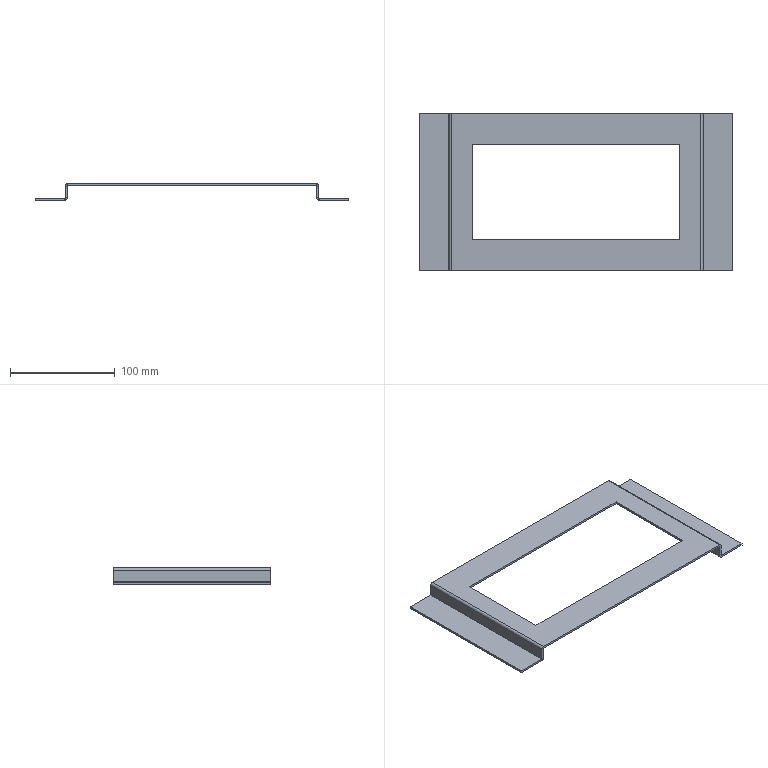Part | 1 solid | 42 faces | box 298 x 150 x 15.5 mm | volume 61242 mm3 | plane 34 | cylinder 8 | commonest cylinder face diameters 0.4 x4 4.4 x4
STEP:
#1=CARTESIAN_POINT('',(121.,75.,-2.2));
#2=VERTEX_POINT('',#1);
#3=CARTESIAN_POINT('',(121.,75.,-13.3));
#4=VERTEX_POINT('',#3);
#5=CARTESIAN_POINT('',(121.,75.,-2.));
#6=DIRECTION('',(0.,0.,-1.));
#7=VECTOR('',#6,1000.);
#8=LINE('',#5,#7);
#9=EDGE_CURVE('',#2,#4,#8,.T.);
#10=ORIENTED_EDGE('',*,*,#9,.T.);
#11=CARTESIAN_POINT('',(119.,75.,-13.3));
#12=VERTEX_POINT('',#11);
#13=CARTESIAN_POINT('',(121.,75.,-13.3));
#14=DIRECTION('',(-1.,0.,0.));
#15=VECTOR('',#14,1000.);
#16=LINE('',#13,#15);
#17=EDGE_CURVE('',#4,#12,#16,.T.);
#18=ORIENTED_EDGE('',*,*,#17,.T.);
#19=CARTESIAN_POINT('',(119.,75.,-2.2));
#20=VERTEX_POINT('',#19);
#21=CARTESIAN_POINT('',(119.,75.,0.));
#22=DIRECTION('',(0.,0.,-1.));
#23=VECTOR('',#22,1000.);
#24=LINE('',#21,#23);
#25=EDGE_CURVE('',#20,#12,#24,.T.);
#26=ORIENTED_EDGE('',*,*,#25,.F.);
#27=CARTESIAN_POINT('',(121.,75.,-2.2));
#28=DIRECTION('',(1.,0.,0.));
#29=VECTOR('',#28,1000.);
#30=LINE('',#27,#29);
#31=EDGE_CURVE('',#20,#2,#30,.T.);
#32=ORIENTED_EDGE('',*,*,#31,.T.);
#33=EDGE_LOOP('',(#10,#18,#26,#32));
#34=FACE_OUTER_BOUND('',#33,.T.);
#35=CARTESIAN_POINT('',(121.,75.,-2.));
#36=DIRECTION('',(0.,1.,0.));
#37=DIRECTION('',(0.,0.,1.));
#38=AXIS2_PLACEMENT_3D('',#35,#36,#37);
#39=PLANE('',#38);
#40=ADVANCED_FACE('',(#34),#39,.T.);
#41=CARTESIAN_POINT('',(121.,-75.,-13.3));
#42=VERTEX_POINT('',#41);
#43=CARTESIAN_POINT('',(121.,75.,-13.3));
#44=DIRECTION('',(0.,-1.,0.));
#45=VECTOR('',#44,1000.);
#46=LINE('',#43,#45);
#47=EDGE_CURVE('',#4,#42,#46,.T.);
#48=ORIENTED_EDGE('',*,*,#47,.F.);
#49=ORIENTED_EDGE('',*,*,#9,.F.);
#50=CARTESIAN_POINT('',(121.,-75.,-2.2));
#51=VERTEX_POINT('',#50);
#52=CARTESIAN_POINT('',(121.,75.,-2.2));
#53=DIRECTION('',(0.,1.,0.));
#54=VECTOR('',#53,1000.);
#55=LINE('',#52,#54);
#56=EDGE_CURVE('',#51,#2,#55,.T.);
#57=ORIENTED_EDGE('',*,*,#56,.F.);
#58=CARTESIAN_POINT('',(121.,-75.,-15.5));
#59=DIRECTION('',(0.,0.,1.));
#60=VECTOR('',#59,1000.);
#61=LINE('',#58,#60);
#62=EDGE_CURVE('',#42,#51,#61,.T.);
#63=ORIENTED_EDGE('',*,*,#62,.F.);
#64=EDGE_LOOP('',(#48,#49,#57,#63));
#65=FACE_OUTER_BOUND('',#64,.T.);
#66=CARTESIAN_POINT('',(121.,0.,0.));
#67=DIRECTION('',(-1.,0.,0.));
#68=DIRECTION('',(0.,0.,1.));
#69=AXIS2_PLACEMENT_3D('',#66,#67,#68);
#70=PLANE('',#69);
#71=ADVANCED_FACE('',(#65),#70,.F.);
#72=ORIENTED_EDGE('',*,*,#25,.T.);
#73=CARTESIAN_POINT('',(119.,-75.,-13.3));
#74=VERTEX_POINT('',#73);
#75=CARTESIAN_POINT('',(119.,75.,-13.3));
#76=DIRECTION('',(0.,-1.,0.));
#77=VECTOR('',#76,1000.);
#78=LINE('',#75,#77);
#79=EDGE_CURVE('',#12,#74,#78,.T.);
#80=ORIENTED_EDGE('',*,*,#79,.T.);
#81=CARTESIAN_POINT('',(119.,-75.,-2.2));
#82=VERTEX_POINT('',#81);
#83=CARTESIAN_POINT('',(119.,-75.,0.));
#84=DIRECTION('',(0.,0.,1.));
#85=VECTOR('',#84,1000.);
#86=LINE('',#83,#85);
#87=EDGE_CURVE('',#74,#82,#86,.T.);
#88=ORIENTED_EDGE('',*,*,#87,.T.);
#89=CARTESIAN_POINT('',(119.,75.,-2.2));
#90=DIRECTION('',(0.,-1.,0.));
#91=VECTOR('',#90,1000.);
#92=LINE('',#89,#91);
#93=EDGE_CURVE('',#20,#82,#92,.T.);
#94=ORIENTED_EDGE('',*,*,#93,.F.);
#95=EDGE_LOOP('',(#72,#80,#88,#94));
#96=FACE_OUTER_BOUND('',#95,.T.);
#97=CARTESIAN_POINT('',(119.,0.,0.));
#98=DIRECTION('',(-1.,0.,0.));
#99=DIRECTION('',(0.,0.,1.));
#100=AXIS2_PLACEMENT_3D('',#97,#98,#99);
#101=PLANE('',#100);
#102=ADVANCED_FACE('',(#96),#101,.T.);
#103=CARTESIAN_POINT('',(-121.,-75.,-2.2));
#104=VERTEX_POINT('',#103);
#105=CARTESIAN_POINT('',(-121.,-75.,-13.3));
#106=VERTEX_POINT('',#105);
#107=CARTESIAN_POINT('',(-121.,-75.,-15.5));
#108=DIRECTION('',(0.,0.,-1.));
#109=VECTOR('',#108,1000.);
#110=LINE('',#107,#109);
#111=EDGE_CURVE('',#104,#106,#110,.T.);
#112=ORIENTED_EDGE('',*,*,#111,.T.);
#113=CARTESIAN_POINT('',(-119.,-75.,-13.3));
#114=VERTEX_POINT('',#113);
#115=CARTESIAN_POINT('',(-121.,-75.,-13.3));
#116=DIRECTION('',(1.,0.,0.));
#117=VECTOR('',#116,1000.);
#118=LINE('',#115,#117);
#119=EDGE_CURVE('',#106,#114,#118,.T.);
#120=ORIENTED_EDGE('',*,*,#119,.T.);
#121=CARTESIAN_POINT('',(-119.,-75.,-2.2));
#122=VERTEX_POINT('',#121);
#123=CARTESIAN_POINT('',(-119.,-75.,0.));
#124=DIRECTION('',(0.,0.,-1.));
#125=VECTOR('',#124,1000.);
#126=LINE('',#123,#125);
#127=EDGE_CURVE('',#122,#114,#126,.T.);
#128=ORIENTED_EDGE('',*,*,#127,.F.);
#129=CARTESIAN_POINT('',(-121.,-75.,-2.2));
#130=DIRECTION('',(-1.,0.,0.));
#131=VECTOR('',#130,1000.);
#132=LINE('',#129,#131);
#133=EDGE_CURVE('',#122,#104,#132,.T.);
#134=ORIENTED_EDGE('',*,*,#133,.T.);
#135=EDGE_LOOP('',(#112,#120,#128,#134));
#136=FACE_OUTER_BOUND('',#135,.T.);
#137=CARTESIAN_POINT('',(-121.,-75.,-15.5));
#138=DIRECTION('',(0.,-1.,0.));
#139=DIRECTION('',(0.,0.,-1.));
#140=AXIS2_PLACEMENT_3D('',#137,#138,#139);
#141=PLANE('',#140);
#142=ADVANCED_FACE('',(#136),#141,.T.);
#143=CARTESIAN_POINT('',(-121.,75.,-13.3));
#144=VERTEX_POINT('',#143);
#145=CARTESIAN_POINT('',(-121.,75.,-2.2));
#146=VERTEX_POINT('',#145);
#147=CARTESIAN_POINT('',(-121.,75.,-2.));
#148=DIRECTION('',(0.,0.,1.));
#149=VECTOR('',#148,1000.);
#150=LINE('',#147,#149);
#151=EDGE_CURVE('',#144,#146,#150,.T.);
#152=ORIENTED_EDGE('',*,*,#151,.F.);
#153=CARTESIAN_POINT('',(-121.,-75.,-13.3));
#154=DIRECTION('',(0.,1.,0.));
#155=VECTOR('',#154,1000.);
#156=LINE('',#153,#155);
#157=EDGE_CURVE('',#106,#144,#156,.T.);
#158=ORIENTED_EDGE('',*,*,#157,.F.);
#159=ORIENTED_EDGE('',*,*,#111,.F.);
#160=CARTESIAN_POINT('',(-121.,0.,-2.2));
#161=DIRECTION('',(0.,1.,0.));
#162=VECTOR('',#161,1000.);
#163=LINE('',#160,#162);
#164=EDGE_CURVE('',#104,#146,#163,.T.);
#165=ORIENTED_EDGE('',*,*,#164,.T.);
#166=EDGE_LOOP('',(#152,#158,#159,#165));
#167=FACE_OUTER_BOUND('',#166,.T.);
#168=CARTESIAN_POINT('',(-121.,0.,0.));
#169=DIRECTION('',(-1.,0.,0.));
#170=DIRECTION('',(0.,0.,1.));
#171=AXIS2_PLACEMENT_3D('',#168,#169,#170);
#172=PLANE('',#171);
#173=ADVANCED_FACE('',(#167),#172,.T.);
#174=CARTESIAN_POINT('',(-119.,75.,-13.3));
#175=VERTEX_POINT('',#174);
#176=CARTESIAN_POINT('',(-119.,-75.,-13.3));
#177=DIRECTION('',(0.,1.,0.));
#178=VECTOR('',#177,1000.);
#179=LINE('',#176,#178);
#180=EDGE_CURVE('',#114,#175,#179,.T.);
#181=ORIENTED_EDGE('',*,*,#180,.T.);
#182=CARTESIAN_POINT('',(-119.,75.,-2.2));
#183=VERTEX_POINT('',#182);
#184=CARTESIAN_POINT('',(-119.,75.,0.));
#185=DIRECTION('',(0.,0.,1.));
#186=VECTOR('',#185,1000.);
#187=LINE('',#184,#186);
#188=EDGE_CURVE('',#175,#183,#187,.T.);
#189=ORIENTED_EDGE('',*,*,#188,.T.);
#190=CARTESIAN_POINT('',(-119.,-75.,-2.2));
#191=DIRECTION('',(0.,1.,0.));
#192=VECTOR('',#191,1000.);
#193=LINE('',#190,#192);
#194=EDGE_CURVE('',#122,#183,#193,.T.);
#195=ORIENTED_EDGE('',*,*,#194,.F.);
#196=ORIENTED_EDGE('',*,*,#127,.T.);
#197=EDGE_LOOP('',(#181,#189,#195,#196));
#198=FACE_OUTER_BOUND('',#197,.T.);
#199=CARTESIAN_POINT('',(-119.,0.,0.));
#200=DIRECTION('',(-1.,0.,0.));
#201=DIRECTION('',(0.,0.,1.));
#202=AXIS2_PLACEMENT_3D('',#199,#200,#201);
#203=PLANE('',#202);
#204=ADVANCED_FACE('',(#198),#203,.F.);
#205=CARTESIAN_POINT('',(99.,45.,-2.));
#206=VERTEX_POINT('',#205);
#207=CARTESIAN_POINT('',(-99.,45.,-2.));
#208=VERTEX_POINT('',#207);
#209=CARTESIAN_POINT('',(0.,45.,-2.));
#210=DIRECTION('',(-1.,0.,0.));
#211=VECTOR('',#210,1000.);
#212=LINE('',#209,#211);
#213=EDGE_CURVE('',#206,#208,#212,.T.);
#214=ORIENTED_EDGE('',*,*,#213,.T.);
#215=CARTESIAN_POINT('',(-99.,-45.,-2.));
#216=VERTEX_POINT('',#215);
#217=CARTESIAN_POINT('',(-99.,0.,-2.));
#218=DIRECTION('',(0.,-1.,0.));
#219=VECTOR('',#218,1000.);
#220=LINE('',#217,#219);
#221=EDGE_CURVE('',#208,#216,#220,.T.);
#222=ORIENTED_EDGE('',*,*,#221,.T.);
#223=CARTESIAN_POINT('',(99.,-45.,-2.));
#224=VERTEX_POINT('',#223);
#225=CARTESIAN_POINT('',(0.,-45.,-2.));
#226=DIRECTION('',(1.,0.,0.));
#227=VECTOR('',#226,1000.);
#228=LINE('',#225,#227);
#229=EDGE_CURVE('',#216,#224,#228,.T.);
#230=ORIENTED_EDGE('',*,*,#229,.T.);
#231=CARTESIAN_POINT('',(99.,0.,-2.));
#232=DIRECTION('',(0.,1.,0.));
#233=VECTOR('',#232,1000.);
#234=LINE('',#231,#233);
#235=EDGE_CURVE('',#224,#206,#234,.T.);
#236=ORIENTED_EDGE('',*,*,#235,.T.);
#237=EDGE_LOOP('',(#214,#222,#230,#236));
#238=FACE_BOUND('',#237,.T.);
#239=CARTESIAN_POINT('',(118.8,-75.,-2.));
#240=VERTEX_POINT('',#239);
#241=CARTESIAN_POINT('',(118.8,75.,-2.));
#242=VERTEX_POINT('',#241);
#243=CARTESIAN_POINT('',(118.8,-75.,-2.));
#244=DIRECTION('',(0.,1.,0.));
#245=VECTOR('',#244,1000.);
#246=LINE('',#243,#245);
#247=EDGE_CURVE('',#240,#242,#246,.T.);
#248=ORIENTED_EDGE('',*,*,#247,.F.);
#249=CARTESIAN_POINT('',(-118.8,-75.,-2.));
#250=VERTEX_POINT('',#249);
#251=CARTESIAN_POINT('',(-121.,-75.,-2.));
#252=DIRECTION('',(1.,0.,0.));
#253=VECTOR('',#252,1000.);
#254=LINE('',#251,#253);
#255=EDGE_CURVE('',#250,#240,#254,.T.);
#256=ORIENTED_EDGE('',*,*,#255,.F.);
#257=CARTESIAN_POINT('',(-118.8,75.,-2.));
#258=VERTEX_POINT('',#257);
#259=CARTESIAN_POINT('',(-118.8,75.,-2.));
#260=DIRECTION('',(0.,-1.,0.));
#261=VECTOR('',#260,1000.);
#262=LINE('',#259,#261);
#263=EDGE_CURVE('',#258,#250,#262,.T.);
#264=ORIENTED_EDGE('',*,*,#263,.F.);
#265=CARTESIAN_POINT('',(-121.,75.,-2.));
#266=DIRECTION('',(-1.,0.,0.));
#267=VECTOR('',#266,1000.);
#268=LINE('',#265,#267);
#269=EDGE_CURVE('',#242,#258,#268,.T.);
#270=ORIENTED_EDGE('',*,*,#269,.F.);
#271=EDGE_LOOP('',(#248,#256,#264,#270));
#272=FACE_OUTER_BOUND('',#271,.T.);
#273=CARTESIAN_POINT('',(0.,0.,-2.));
#274=DIRECTION('',(0.,0.,1.));
#275=DIRECTION('',(1.,0.,0.));
#276=AXIS2_PLACEMENT_3D('',#273,#274,#275);
#277=PLANE('',#276);
#278=ADVANCED_FACE('',(#238,#272),#277,.F.);
#279=CARTESIAN_POINT('',(-99.,45.,0.));
#280=VERTEX_POINT('',#279);
#281=CARTESIAN_POINT('',(-99.,-45.,0.));
#282=VERTEX_POINT('',#281);
#283=CARTESIAN_POINT('',(-99.,45.,0.));
#284=DIRECTION('',(0.,-1.,0.));
#285=VECTOR('',#284,1000.);
#286=LINE('',#283,#285);
#287=EDGE_CURVE('',#280,#282,#286,.T.);
#288=ORIENTED_EDGE('',*,*,#287,.F.);
#289=CARTESIAN_POINT('',(99.,45.,0.));
#290=VERTEX_POINT('',#289);
#291=CARTESIAN_POINT('',(99.,45.,0.));
#292=DIRECTION('',(-1.,0.,0.));
#293=VECTOR('',#292,1000.);
#294=LINE('',#291,#293);
#295=EDGE_CURVE('',#290,#280,#294,.T.);
#296=ORIENTED_EDGE('',*,*,#295,.F.);
#297=CARTESIAN_POINT('',(99.,-45.,0.));
#298=VERTEX_POINT('',#297);
#299=CARTESIAN_POINT('',(99.,45.,0.));
#300=DIRECTION('',(0.,1.,0.));
#301=VECTOR('',#300,1000.);
#302=LINE('',#299,#301);
#303=EDGE_CURVE('',#298,#290,#302,.T.);
#304=ORIENTED_EDGE('',*,*,#303,.F.);
#305=CARTESIAN_POINT('',(99.,-45.,0.));
#306=DIRECTION('',(1.,0.,0.));
#307=VECTOR('',#306,1000.);
#308=LINE('',#305,#307);
#309=EDGE_CURVE('',#282,#298,#308,.T.);
#310=ORIENTED_EDGE('',*,*,#309,.F.);
#311=EDGE_LOOP('',(#288,#296,#304,#310));
#312=FACE_BOUND('',#311,.T.);
#313=CARTESIAN_POINT('',(-118.8,-75.,0.));
#314=VERTEX_POINT('',#313);
#315=CARTESIAN_POINT('',(118.8,-75.,0.));
#316=VERTEX_POINT('',#315);
#317=CARTESIAN_POINT('',(-121.,-75.,0.));
#318=DIRECTION('',(1.,0.,0.));
#319=VECTOR('',#318,1000.);
#320=LINE('',#317,#319);
#321=EDGE_CURVE('',#314,#316,#320,.T.);
#322=ORIENTED_EDGE('',*,*,#321,.T.);
#323=CARTESIAN_POINT('',(118.8,75.,0.));
#324=VERTEX_POINT('',#323);
#325=CARTESIAN_POINT('',(118.8,-75.,0.));
#326=DIRECTION('',(0.,1.,0.));
#327=VECTOR('',#326,1000.);
#328=LINE('',#325,#327);
#329=EDGE_CURVE('',#316,#324,#328,.T.);
#330=ORIENTED_EDGE('',*,*,#329,.T.);
#331=CARTESIAN_POINT('',(-118.8,75.,0.));
#332=VERTEX_POINT('',#331);
#333=CARTESIAN_POINT('',(-121.,75.,0.));
#334=DIRECTION('',(-1.,0.,0.));
#335=VECTOR('',#334,1000.);
#336=LINE('',#333,#335);
#337=EDGE_CURVE('',#324,#332,#336,.T.);
#338=ORIENTED_EDGE('',*,*,#337,.T.);
#339=CARTESIAN_POINT('',(-118.8,75.,0.));
#340=DIRECTION('',(0.,-1.,0.));
#341=VECTOR('',#340,1000.);
#342=LINE('',#339,#341);
#343=EDGE_CURVE('',#332,#314,#342,.T.);
#344=ORIENTED_EDGE('',*,*,#343,.T.);
#345=EDGE_LOOP('',(#322,#330,#338,#344));
#346=FACE_OUTER_BOUND('',#345,.T.);
#347=CARTESIAN_POINT('',(0.,0.,0.));
#348=DIRECTION('',(0.,0.,1.));
#349=DIRECTION('',(1.,0.,0.));
#350=AXIS2_PLACEMENT_3D('',#347,#348,#349);
#351=PLANE('',#350);
#352=ADVANCED_FACE('',(#312,#346),#351,.T.);
#353=ORIENTED_EDGE('',*,*,#255,.T.);
#354=CARTESIAN_POINT('',(118.8,-75.,-2.));
#355=DIRECTION('',(0.,0.,1.));
#356=VECTOR('',#355,1000.);
#357=LINE('',#354,#356);
#358=EDGE_CURVE('',#240,#316,#357,.T.);
#359=ORIENTED_EDGE('',*,*,#358,.T.);
#360=ORIENTED_EDGE('',*,*,#321,.F.);
#361=CARTESIAN_POINT('',(-118.8,-75.,-2.));
#362=DIRECTION('',(0.,0.,1.));
#363=VECTOR('',#362,1000.);
#364=LINE('',#361,#363);
#365=EDGE_CURVE('',#250,#314,#364,.T.);
#366=ORIENTED_EDGE('',*,*,#365,.F.);
#367=EDGE_LOOP('',(#353,#359,#360,#366));
#368=FACE_OUTER_BOUND('',#367,.T.);
#369=CARTESIAN_POINT('',(-121.,-75.,-2.));
#370=DIRECTION('',(0.,-1.,0.));
#371=DIRECTION('',(0.,0.,-1.));
#372=AXIS2_PLACEMENT_3D('',#369,#370,#371);
#373=PLANE('',#372);
#374=ADVANCED_FACE('',(#368),#373,.T.);
#375=CARTESIAN_POINT('',(118.8,75.,-2.));
#376=DIRECTION('',(0.,0.,1.));
#377=VECTOR('',#376,1000.);
#378=LINE('',#375,#377);
#379=EDGE_CURVE('',#242,#324,#378,.T.);
#380=ORIENTED_EDGE('',*,*,#379,.F.);
#381=ORIENTED_EDGE('',*,*,#269,.T.);
#382=CARTESIAN_POINT('',(-118.8,75.,-2.));
#383=DIRECTION('',(0.,0.,1.));
#384=VECTOR('',#383,1000.);
#385=LINE('',#382,#384);
#386=EDGE_CURVE('',#258,#332,#385,.T.);
#387=ORIENTED_EDGE('',*,*,#386,.T.);
#388=ORIENTED_EDGE('',*,*,#337,.F.);
#389=EDGE_LOOP('',(#380,#381,#387,#388));
#390=FACE_OUTER_BOUND('',#389,.T.);
#391=CARTESIAN_POINT('',(-121.,75.,-2.));
#392=DIRECTION('',(0.,1.,0.));
#393=DIRECTION('',(0.,0.,1.));
#394=AXIS2_PLACEMENT_3D('',#391,#392,#393);
#395=PLANE('',#394);
#396=ADVANCED_FACE('',(#390),#395,.T.);
#397=ORIENTED_EDGE('',*,*,#133,.F.);
#398=CARTESIAN_POINT('',(-118.8,-75.,-2.2));
#399=DIRECTION('',(0.,-1.,0.));
#400=DIRECTION('',(0.,0.,1.));
#401=AXIS2_PLACEMENT_3D('',#398,#399,#400);
#402=CIRCLE('',#401,0.2);
#403=EDGE_CURVE('',#250,#122,#402,.T.);
#404=ORIENTED_EDGE('',*,*,#403,.F.);
#405=ORIENTED_EDGE('',*,*,#365,.T.);
#406=CARTESIAN_POINT('',(-118.8,-75.,-2.2));
#407=DIRECTION('',(0.,-1.,0.));
#408=DIRECTION('',(0.,0.,1.));
#409=AXIS2_PLACEMENT_3D('',#406,#407,#408);
#410=CIRCLE('',#409,2.2);
#411=EDGE_CURVE('',#314,#104,#410,.T.);
#412=ORIENTED_EDGE('',*,*,#411,.T.);
#413=EDGE_LOOP('',(#397,#404,#405,#412));
#414=FACE_OUTER_BOUND('',#413,.T.);
#415=CARTESIAN_POINT('',(-118.8,-75.,-2.2));
#416=DIRECTION('',(0.,-1.,0.));
#417=DIRECTION('',(0.,0.,-1.));
#418=AXIS2_PLACEMENT_3D('',#415,#416,#417);
#419=PLANE('',#418);
#420=ADVANCED_FACE('',(#414),#419,.T.);
#421=CARTESIAN_POINT('',(-118.8,75.,-2.2));
#422=DIRECTION('',(0.,1.,0.));
#423=DIRECTION('',(0.,0.,1.));
#424=AXIS2_PLACEMENT_3D('',#421,#422,#423);
#425=CIRCLE('',#424,0.2);
#426=EDGE_CURVE('',#183,#258,#425,.T.);
#427=ORIENTED_EDGE('',*,*,#426,.F.);
#428=CARTESIAN_POINT('',(-119.,75.,-2.2));
#429=DIRECTION('',(-1.,0.,0.));
#430=VECTOR('',#429,1000.);
#431=LINE('',#428,#430);
#432=EDGE_CURVE('',#183,#146,#431,.T.);
#433=ORIENTED_EDGE('',*,*,#432,.T.);
#434=CARTESIAN_POINT('',(-118.8,75.,-2.2));
#435=DIRECTION('',(0.,1.,0.));
#436=DIRECTION('',(0.,0.,1.));
#437=AXIS2_PLACEMENT_3D('',#434,#435,#436);
#438=CIRCLE('',#437,2.2);
#439=EDGE_CURVE('',#146,#332,#438,.T.);
#440=ORIENTED_EDGE('',*,*,#439,.T.);
#441=ORIENTED_EDGE('',*,*,#386,.F.);
#442=EDGE_LOOP('',(#427,#433,#440,#441));
#443=FACE_OUTER_BOUND('',#442,.T.);
#444=CARTESIAN_POINT('',(-118.8,75.,-2.2));
#445=DIRECTION('',(0.,-1.,0.));
#446=DIRECTION('',(0.,0.,-1.));
#447=AXIS2_PLACEMENT_3D('',#444,#445,#446);
#448=PLANE('',#447);
#449=ADVANCED_FACE('',(#443),#448,.F.);
#450=ORIENTED_EDGE('',*,*,#343,.F.);
#451=ORIENTED_EDGE('',*,*,#439,.F.);
#452=ORIENTED_EDGE('',*,*,#164,.F.);
#453=ORIENTED_EDGE('',*,*,#411,.F.);
#454=EDGE_LOOP('',(#450,#451,#452,#453));
#455=FACE_OUTER_BOUND('',#454,.T.);
#456=CARTESIAN_POINT('',(-118.8,75.,-2.2));
#457=DIRECTION('',(0.,1.,0.));
#458=DIRECTION('',(-1.,0.,0.));
#459=AXIS2_PLACEMENT_3D('',#456,#457,#458);
#460=CYLINDRICAL_SURFACE('',#459,2.2);
#461=ADVANCED_FACE('',(#455),#460,.T.);
#462=ORIENTED_EDGE('',*,*,#263,.T.);
#463=ORIENTED_EDGE('',*,*,#403,.T.);
#464=ORIENTED_EDGE('',*,*,#194,.T.);
#465=ORIENTED_EDGE('',*,*,#426,.T.);
#466=EDGE_LOOP('',(#462,#463,#464,#465));
#467=FACE_OUTER_BOUND('',#466,.T.);
#468=CARTESIAN_POINT('',(-118.8,75.,-2.2));
#469=DIRECTION('',(0.,1.,0.));
#470=DIRECTION('',(-1.,0.,0.));
#471=AXIS2_PLACEMENT_3D('',#468,#469,#470);
#472=CYLINDRICAL_SURFACE('',#471,0.2);
#473=ADVANCED_FACE('',(#467),#472,.F.);
#474=CARTESIAN_POINT('',(-121.,75.,-13.3));
#475=DIRECTION('',(1.,0.,0.));
#476=VECTOR('',#475,1000.);
#477=LINE('',#474,#476);
#478=EDGE_CURVE('',#144,#175,#477,.T.);
#479=ORIENTED_EDGE('',*,*,#478,.F.);
#480=ORIENTED_EDGE('',*,*,#151,.T.);
#481=ORIENTED_EDGE('',*,*,#432,.F.);
#482=ORIENTED_EDGE('',*,*,#188,.F.);
#483=EDGE_LOOP('',(#479,#480,#481,#482));
#484=FACE_OUTER_BOUND('',#483,.T.);
#485=CARTESIAN_POINT('',(-121.,75.,-2.));
#486=DIRECTION('',(0.,1.,0.));
#487=DIRECTION('',(0.,0.,1.));
#488=AXIS2_PLACEMENT_3D('',#485,#486,#487);
#489=PLANE('',#488);
#490=ADVANCED_FACE('',(#484),#489,.T.);
#491=ORIENTED_EDGE('',*,*,#31,.F.);
#492=CARTESIAN_POINT('',(118.8,75.,-2.2));
#493=DIRECTION('',(0.,1.,0.));
#494=DIRECTION('',(0.,0.,-1.));
#495=AXIS2_PLACEMENT_3D('',#492,#493,#494);
#496=CIRCLE('',#495,0.2);
#497=EDGE_CURVE('',#242,#20,#496,.T.);
#498=ORIENTED_EDGE('',*,*,#497,.F.);
#499=ORIENTED_EDGE('',*,*,#379,.T.);
#500=CARTESIAN_POINT('',(118.8,75.,-2.2));
#501=DIRECTION('',(0.,1.,0.));
#502=DIRECTION('',(0.,0.,-1.));
#503=AXIS2_PLACEMENT_3D('',#500,#501,#502);
#504=CIRCLE('',#503,2.2);
#505=EDGE_CURVE('',#324,#2,#504,.T.);
#506=ORIENTED_EDGE('',*,*,#505,.T.);
#507=EDGE_LOOP('',(#491,#498,#499,#506));
#508=FACE_OUTER_BOUND('',#507,.T.);
#509=CARTESIAN_POINT('',(118.8,75.,-2.2));
#510=DIRECTION('',(0.,1.,0.));
#511=DIRECTION('',(0.,0.,1.));
#512=AXIS2_PLACEMENT_3D('',#509,#510,#511);
#513=PLANE('',#512);
#514=ADVANCED_FACE('',(#508),#513,.T.);
#515=CARTESIAN_POINT('',(118.8,-75.,-2.2));
#516=DIRECTION('',(0.,-1.,0.));
#517=DIRECTION('',(0.,0.,-1.));
#518=AXIS2_PLACEMENT_3D('',#515,#516,#517);
#519=CIRCLE('',#518,0.2);
#520=EDGE_CURVE('',#82,#240,#519,.T.);
#521=ORIENTED_EDGE('',*,*,#520,.F.);
#522=CARTESIAN_POINT('',(119.,-75.,-2.2));
#523=DIRECTION('',(1.,0.,0.));
#524=VECTOR('',#523,1000.);
#525=LINE('',#522,#524);
#526=EDGE_CURVE('',#82,#51,#525,.T.);
#527=ORIENTED_EDGE('',*,*,#526,.T.);
#528=CARTESIAN_POINT('',(118.8,-75.,-2.2));
#529=DIRECTION('',(0.,-1.,0.));
#530=DIRECTION('',(0.,0.,-1.));
#531=AXIS2_PLACEMENT_3D('',#528,#529,#530);
#532=CIRCLE('',#531,2.2);
#533=EDGE_CURVE('',#51,#316,#532,.T.);
#534=ORIENTED_EDGE('',*,*,#533,.T.);
#535=ORIENTED_EDGE('',*,*,#358,.F.);
#536=EDGE_LOOP('',(#521,#527,#534,#535));
#537=FACE_OUTER_BOUND('',#536,.T.);
#538=CARTESIAN_POINT('',(118.8,-75.,-2.2));
#539=DIRECTION('',(0.,1.,0.));
#540=DIRECTION('',(0.,0.,1.));
#541=AXIS2_PLACEMENT_3D('',#538,#539,#540);
#542=PLANE('',#541);
#543=ADVANCED_FACE('',(#537),#542,.F.);
#544=ORIENTED_EDGE('',*,*,#329,.F.);
#545=ORIENTED_EDGE('',*,*,#533,.F.);
#546=ORIENTED_EDGE('',*,*,#56,.T.);
#547=ORIENTED_EDGE('',*,*,#505,.F.);
#548=EDGE_LOOP('',(#544,#545,#546,#547));
#549=FACE_OUTER_BOUND('',#548,.T.);
#550=CARTESIAN_POINT('',(118.8,-75.,-2.2));
#551=DIRECTION('',(0.,-1.,0.));
#552=DIRECTION('',(1.,0.,0.));
#553=AXIS2_PLACEMENT_3D('',#550,#551,#552);
#554=CYLINDRICAL_SURFACE('',#553,2.2);
#555=ADVANCED_FACE('',(#549),#554,.T.);
#556=ORIENTED_EDGE('',*,*,#247,.T.);
#557=ORIENTED_EDGE('',*,*,#497,.T.);
#558=ORIENTED_EDGE('',*,*,#93,.T.);
#559=ORIENTED_EDGE('',*,*,#520,.T.);
#560=EDGE_LOOP('',(#556,#557,#558,#559));
#561=FACE_OUTER_BOUND('',#560,.T.);
#562=CARTESIAN_POINT('',(118.8,-75.,-2.2));
#563=DIRECTION('',(0.,-1.,0.));
#564=DIRECTION('',(1.,0.,0.));
#565=AXIS2_PLACEMENT_3D('',#562,#563,#564);
#566=CYLINDRICAL_SURFACE('',#565,0.2);
#567=ADVANCED_FACE('',(#561),#566,.F.);
#568=CARTESIAN_POINT('',(121.,-75.,-13.3));
#569=DIRECTION('',(-1.,0.,0.));
#570=VECTOR('',#569,1000.);
#571=LINE('',#568,#570);
#572=EDGE_CURVE('',#42,#74,#571,.T.);
#573=ORIENTED_EDGE('',*,*,#572,.F.);
#574=ORIENTED_EDGE('',*,*,#62,.T.);
#575=ORIENTED_EDGE('',*,*,#526,.F.);
#576=ORIENTED_EDGE('',*,*,#87,.F.);
#577=EDGE_LOOP('',(#573,#574,#575,#576));
#578=FACE_OUTER_BOUND('',#577,.T.);
#579=CARTESIAN_POINT('',(121.,-75.,-15.5));
#580=DIRECTION('',(0.,-1.,0.));
#581=DIRECTION('',(0.,0.,-1.));
#582=AXIS2_PLACEMENT_3D('',#579,#580,#581);
#583=PLANE('',#582);
#584=ADVANCED_FACE('',(#578),#583,.T.);
#585=CARTESIAN_POINT('',(-121.2,75.,-13.5));
#586=VERTEX_POINT('',#585);
#587=CARTESIAN_POINT('',(-121.2,75.,-15.5));
#588=VERTEX_POINT('',#587);
#589=CARTESIAN_POINT('',(-121.2,75.,-15.5));
#590=DIRECTION('',(0.,0.,-1.));
#591=VECTOR('',#590,1000.);
#592=LINE('',#589,#591);
#593=EDGE_CURVE('',#586,#588,#592,.T.);
#594=ORIENTED_EDGE('',*,*,#593,.F.);
#595=CARTESIAN_POINT('',(-121.2,75.,-13.3));
#596=DIRECTION('',(0.,1.,0.));
#597=DIRECTION('',(0.,0.,-1.));
#598=AXIS2_PLACEMENT_3D('',#595,#596,#597);
#599=CIRCLE('',#598,0.2);
#600=EDGE_CURVE('',#144,#586,#599,.T.);
#601=ORIENTED_EDGE('',*,*,#600,.F.);
#602=ORIENTED_EDGE('',*,*,#478,.T.);
#603=CARTESIAN_POINT('',(-121.2,75.,-13.3));
#604=DIRECTION('',(0.,1.,0.));
#605=DIRECTION('',(0.,0.,-1.));
#606=AXIS2_PLACEMENT_3D('',#603,#604,#605);
#607=CIRCLE('',#606,2.2);
#608=EDGE_CURVE('',#175,#588,#607,.T.);
#609=ORIENTED_EDGE('',*,*,#608,.T.);
#610=EDGE_LOOP('',(#594,#601,#602,#609));
#611=FACE_OUTER_BOUND('',#610,.T.);
#612=CARTESIAN_POINT('',(-121.2,75.,-13.3));
#613=DIRECTION('',(0.,1.,0.));
#614=DIRECTION('',(0.,0.,1.));
#615=AXIS2_PLACEMENT_3D('',#612,#613,#614);
#616=PLANE('',#615);
#617=ADVANCED_FACE('',(#611),#616,.T.);
#618=CARTESIAN_POINT('',(-121.2,-75.,-13.5));
#619=VERTEX_POINT('',#618);
#620=CARTESIAN_POINT('',(-121.2,-75.,-13.3));
#621=DIRECTION('',(0.,-1.,0.));
#622=DIRECTION('',(0.,0.,-1.));
#623=AXIS2_PLACEMENT_3D('',#620,#621,#622);
#624=CIRCLE('',#623,0.2);
#625=EDGE_CURVE('',#619,#106,#624,.T.);
#626=ORIENTED_EDGE('',*,*,#625,.F.);
#627=CARTESIAN_POINT('',(-121.2,-75.,-15.5));
#628=VERTEX_POINT('',#627);
#629=CARTESIAN_POINT('',(-121.2,-75.,-13.5));
#630=DIRECTION('',(0.,0.,-1.));
#631=VECTOR('',#630,1000.);
#632=LINE('',#629,#631);
#633=EDGE_CURVE('',#619,#628,#632,.T.);
#634=ORIENTED_EDGE('',*,*,#633,.T.);
#635=CARTESIAN_POINT('',(-121.2,-75.,-13.3));
#636=DIRECTION('',(0.,-1.,0.));
#637=DIRECTION('',(0.,0.,-1.));
#638=AXIS2_PLACEMENT_3D('',#635,#636,#637);
#639=CIRCLE('',#638,2.2);
#640=EDGE_CURVE('',#628,#114,#639,.T.);
#641=ORIENTED_EDGE('',*,*,#640,.T.);
#642=ORIENTED_EDGE('',*,*,#119,.F.);
#643=EDGE_LOOP('',(#626,#634,#641,#642));
#644=FACE_OUTER_BOUND('',#643,.T.);
#645=CARTESIAN_POINT('',(-121.2,-75.,-13.3));
#646=DIRECTION('',(0.,1.,0.));
#647=DIRECTION('',(0.,0.,1.));
#648=AXIS2_PLACEMENT_3D('',#645,#646,#647);
#649=PLANE('',#648);
#650=ADVANCED_FACE('',(#644),#649,.F.);
#651=ORIENTED_EDGE('',*,*,#180,.F.);
#652=ORIENTED_EDGE('',*,*,#640,.F.);
#653=CARTESIAN_POINT('',(-121.2,75.,-15.5));
#654=DIRECTION('',(0.,1.,0.));
#655=VECTOR('',#654,1000.);
#656=LINE('',#653,#655);
#657=EDGE_CURVE('',#628,#588,#656,.T.);
#658=ORIENTED_EDGE('',*,*,#657,.T.);
#659=ORIENTED_EDGE('',*,*,#608,.F.);
#660=EDGE_LOOP('',(#651,#652,#658,#659));
#661=FACE_OUTER_BOUND('',#660,.T.);
#662=CARTESIAN_POINT('',(-121.2,-75.,-13.3));
#663=DIRECTION('',(0.,-1.,0.));
#664=DIRECTION('',(0.,0.,-1.));
#665=AXIS2_PLACEMENT_3D('',#662,#663,#664);
#666=CYLINDRICAL_SURFACE('',#665,2.2);
#667=ADVANCED_FACE('',(#661),#666,.T.);
#668=ORIENTED_EDGE('',*,*,#157,.T.);
#669=ORIENTED_EDGE('',*,*,#600,.T.);
#670=CARTESIAN_POINT('',(-121.2,75.,-13.5));
#671=DIRECTION('',(0.,-1.,0.));
#672=VECTOR('',#671,1000.);
#673=LINE('',#670,#672);
#674=EDGE_CURVE('',#586,#619,#673,.T.);
#675=ORIENTED_EDGE('',*,*,#674,.T.);
#676=ORIENTED_EDGE('',*,*,#625,.T.);
#677=EDGE_LOOP('',(#668,#669,#675,#676));
#678=FACE_OUTER_BOUND('',#677,.T.);
#679=CARTESIAN_POINT('',(-121.2,-75.,-13.3));
#680=DIRECTION('',(0.,-1.,0.));
#681=DIRECTION('',(0.,0.,-1.));
#682=AXIS2_PLACEMENT_3D('',#679,#680,#681);
#683=CYLINDRICAL_SURFACE('',#682,0.2);
#684=ADVANCED_FACE('',(#678),#683,.F.);
#685=ORIENTED_EDGE('',*,*,#633,.F.);
#686=CARTESIAN_POINT('',(-149.,-75.,-13.5));
#687=VERTEX_POINT('',#686);
#688=CARTESIAN_POINT('',(-149.,-75.,-13.5));
#689=DIRECTION('',(-1.,0.,0.));
#690=VECTOR('',#689,1000.);
#691=LINE('',#688,#690);
#692=EDGE_CURVE('',#619,#687,#691,.T.);
#693=ORIENTED_EDGE('',*,*,#692,.T.);
#694=CARTESIAN_POINT('',(-149.,-75.,-15.5));
#695=VERTEX_POINT('',#694);
#696=CARTESIAN_POINT('',(-149.,-75.,-15.5));
#697=DIRECTION('',(0.,0.,1.));
#698=VECTOR('',#697,1000.);
#699=LINE('',#696,#698);
#700=EDGE_CURVE('',#695,#687,#699,.T.);
#701=ORIENTED_EDGE('',*,*,#700,.F.);
#702=CARTESIAN_POINT('',(0.,-75.,-15.5));
#703=DIRECTION('',(-1.,0.,0.));
#704=VECTOR('',#703,1000.);
#705=LINE('',#702,#704);
#706=EDGE_CURVE('',#628,#695,#705,.T.);
#707=ORIENTED_EDGE('',*,*,#706,.F.);
#708=EDGE_LOOP('',(#685,#693,#701,#707));
#709=FACE_OUTER_BOUND('',#708,.T.);
#710=CARTESIAN_POINT('',(-149.,-75.,-15.5));
#711=DIRECTION('',(0.,1.,0.));
#712=DIRECTION('',(-1.,0.,0.));
#713=AXIS2_PLACEMENT_3D('',#710,#711,#712);
#714=PLANE('',#713);
#715=ADVANCED_FACE('',(#709),#714,.F.);
#716=ORIENTED_EDGE('',*,*,#593,.T.);
#717=CARTESIAN_POINT('',(-149.,75.,-15.5));
#718=VERTEX_POINT('',#717);
#719=CARTESIAN_POINT('',(0.,75.,-15.5));
#720=DIRECTION('',(1.,0.,0.));
#721=VECTOR('',#720,1000.);
#722=LINE('',#719,#721);
#723=EDGE_CURVE('',#718,#588,#722,.T.);
#724=ORIENTED_EDGE('',*,*,#723,.F.);
#725=CARTESIAN_POINT('',(-149.,75.,-13.5));
#726=VERTEX_POINT('',#725);
#727=CARTESIAN_POINT('',(-149.,75.,-15.5));
#728=DIRECTION('',(0.,0.,1.));
#729=VECTOR('',#728,1000.);
#730=LINE('',#727,#729);
#731=EDGE_CURVE('',#718,#726,#730,.T.);
#732=ORIENTED_EDGE('',*,*,#731,.T.);
#733=CARTESIAN_POINT('',(-121.,75.,-13.5));
#734=DIRECTION('',(1.,0.,0.));
#735=VECTOR('',#734,1000.);
#736=LINE('',#733,#735);
#737=EDGE_CURVE('',#726,#586,#736,.T.);
#738=ORIENTED_EDGE('',*,*,#737,.T.);
#739=EDGE_LOOP('',(#716,#724,#732,#738));
#740=FACE_OUTER_BOUND('',#739,.T.);
#741=CARTESIAN_POINT('',(-121.,75.,-15.5));
#742=DIRECTION('',(0.,-1.,0.));
#743=DIRECTION('',(0.,0.,-1.));
#744=AXIS2_PLACEMENT_3D('',#741,#742,#743);
#745=PLANE('',#744);
#746=ADVANCED_FACE('',(#740),#745,.F.);
#747=ORIENTED_EDGE('',*,*,#657,.F.);
#748=ORIENTED_EDGE('',*,*,#706,.T.);
#749=CARTESIAN_POINT('',(-149.,0.,-15.5));
#750=DIRECTION('',(0.,1.,0.));
#751=VECTOR('',#750,1000.);
#752=LINE('',#749,#751);
#753=EDGE_CURVE('',#695,#718,#752,.T.);
#754=ORIENTED_EDGE('',*,*,#753,.T.);
#755=ORIENTED_EDGE('',*,*,#723,.T.);
#756=EDGE_LOOP('',(#747,#748,#754,#755));
#757=FACE_OUTER_BOUND('',#756,.T.);
#758=CARTESIAN_POINT('',(0.,0.,-15.5));
#759=DIRECTION('',(0.,0.,1.));
#760=DIRECTION('',(1.,0.,0.));
#761=AXIS2_PLACEMENT_3D('',#758,#759,#760);
#762=PLANE('',#761);
#763=ADVANCED_FACE('',(#757),#762,.F.);
#764=ORIENTED_EDGE('',*,*,#692,.F.);
#765=ORIENTED_EDGE('',*,*,#674,.F.);
#766=ORIENTED_EDGE('',*,*,#737,.F.);
#767=CARTESIAN_POINT('',(-149.,75.,-13.5));
#768=DIRECTION('',(0.,1.,0.));
#769=VECTOR('',#768,1000.);
#770=LINE('',#767,#769);
#771=EDGE_CURVE('',#687,#726,#770,.T.);
#772=ORIENTED_EDGE('',*,*,#771,.F.);
#773=EDGE_LOOP('',(#764,#765,#766,#772));
#774=FACE_OUTER_BOUND('',#773,.T.);
#775=CARTESIAN_POINT('',(0.,0.,-13.5));
#776=DIRECTION('',(0.,0.,1.));
#777=DIRECTION('',(1.,0.,0.));
#778=AXIS2_PLACEMENT_3D('',#775,#776,#777);
#779=PLANE('',#778);
#780=ADVANCED_FACE('',(#774),#779,.T.);
#781=ORIENTED_EDGE('',*,*,#771,.T.);
#782=ORIENTED_EDGE('',*,*,#731,.F.);
#783=ORIENTED_EDGE('',*,*,#753,.F.);
#784=ORIENTED_EDGE('',*,*,#700,.T.);
#785=EDGE_LOOP('',(#781,#782,#783,#784));
#786=FACE_OUTER_BOUND('',#785,.T.);
#787=CARTESIAN_POINT('',(-149.,75.,-15.5));
#788=DIRECTION('',(1.,0.,0.));
#789=DIRECTION('',(0.,0.,-1.));
#790=AXIS2_PLACEMENT_3D('',#787,#788,#789);
#791=PLANE('',#790);
#792=ADVANCED_FACE('',(#786),#791,.F.);
#793=CARTESIAN_POINT('',(121.2,-75.,-13.5));
#794=VERTEX_POINT('',#793);
#795=CARTESIAN_POINT('',(121.2,-75.,-15.5));
#796=VERTEX_POINT('',#795);
#797=CARTESIAN_POINT('',(121.2,-75.,-15.5));
#798=DIRECTION('',(0.,0.,-1.));
#799=VECTOR('',#798,1000.);
#800=LINE('',#797,#799);
#801=EDGE_CURVE('',#794,#796,#800,.T.);
#802=ORIENTED_EDGE('',*,*,#801,.F.);
#803=CARTESIAN_POINT('',(121.2,-75.,-13.3));
#804=DIRECTION('',(0.,-1.,0.));
#805=DIRECTION('',(0.,0.,1.));
#806=AXIS2_PLACEMENT_3D('',#803,#804,#805);
#807=CIRCLE('',#806,0.2);
#808=EDGE_CURVE('',#42,#794,#807,.T.);
#809=ORIENTED_EDGE('',*,*,#808,.F.);
#810=ORIENTED_EDGE('',*,*,#572,.T.);
#811=CARTESIAN_POINT('',(121.2,-75.,-13.3));
#812=DIRECTION('',(0.,-1.,0.));
#813=DIRECTION('',(0.,0.,1.));
#814=AXIS2_PLACEMENT_3D('',#811,#812,#813);
#815=CIRCLE('',#814,2.2);
#816=EDGE_CURVE('',#74,#796,#815,.T.);
#817=ORIENTED_EDGE('',*,*,#816,.T.);
#818=EDGE_LOOP('',(#802,#809,#810,#817));
#819=FACE_OUTER_BOUND('',#818,.T.);
#820=CARTESIAN_POINT('',(121.2,-75.,-13.3));
#821=DIRECTION('',(0.,-1.,0.));
#822=DIRECTION('',(0.,0.,-1.));
#823=AXIS2_PLACEMENT_3D('',#820,#821,#822);
#824=PLANE('',#823);
#825=ADVANCED_FACE('',(#819),#824,.T.);
#826=CARTESIAN_POINT('',(121.2,75.,-13.5));
#827=VERTEX_POINT('',#826);
#828=CARTESIAN_POINT('',(121.2,75.,-13.3));
#829=DIRECTION('',(0.,1.,0.));
#830=DIRECTION('',(0.,0.,1.));
#831=AXIS2_PLACEMENT_3D('',#828,#829,#830);
#832=CIRCLE('',#831,0.2);
#833=EDGE_CURVE('',#827,#4,#832,.T.);
#834=ORIENTED_EDGE('',*,*,#833,.F.);
#835=CARTESIAN_POINT('',(121.2,75.,-15.5));
#836=VERTEX_POINT('',#835);
#837=CARTESIAN_POINT('',(121.2,75.,-13.5));
#838=DIRECTION('',(0.,0.,-1.));
#839=VECTOR('',#838,1000.);
#840=LINE('',#837,#839);
#841=EDGE_CURVE('',#827,#836,#840,.T.);
#842=ORIENTED_EDGE('',*,*,#841,.T.);
#843=CARTESIAN_POINT('',(121.2,75.,-13.3));
#844=DIRECTION('',(0.,1.,0.));
#845=DIRECTION('',(0.,0.,1.));
#846=AXIS2_PLACEMENT_3D('',#843,#844,#845);
#847=CIRCLE('',#846,2.2);
#848=EDGE_CURVE('',#836,#12,#847,.T.);
#849=ORIENTED_EDGE('',*,*,#848,.T.);
#850=ORIENTED_EDGE('',*,*,#17,.F.);
#851=EDGE_LOOP('',(#834,#842,#849,#850));
#852=FACE_OUTER_BOUND('',#851,.T.);
#853=CARTESIAN_POINT('',(121.2,75.,-13.3));
#854=DIRECTION('',(0.,-1.,0.));
#855=DIRECTION('',(0.,0.,-1.));
#856=AXIS2_PLACEMENT_3D('',#853,#854,#855);
#857=PLANE('',#856);
#858=ADVANCED_FACE('',(#852),#857,.F.);
#859=ORIENTED_EDGE('',*,*,#79,.F.);
#860=ORIENTED_EDGE('',*,*,#848,.F.);
#861=CARTESIAN_POINT('',(121.2,-75.,-15.5));
#862=DIRECTION('',(0.,-1.,0.));
#863=VECTOR('',#862,1000.);
#864=LINE('',#861,#863);
#865=EDGE_CURVE('',#836,#796,#864,.T.);
#866=ORIENTED_EDGE('',*,*,#865,.T.);
#867=ORIENTED_EDGE('',*,*,#816,.F.);
#868=EDGE_LOOP('',(#859,#860,#866,#867));
#869=FACE_OUTER_BOUND('',#868,.T.);
#870=CARTESIAN_POINT('',(121.2,75.,-13.3));
#871=DIRECTION('',(0.,1.,0.));
#872=DIRECTION('',(0.,0.,-1.));
#873=AXIS2_PLACEMENT_3D('',#870,#871,#872);
#874=CYLINDRICAL_SURFACE('',#873,2.2);
#875=ADVANCED_FACE('',(#869),#874,.T.);
#876=ORIENTED_EDGE('',*,*,#47,.T.);
#877=ORIENTED_EDGE('',*,*,#808,.T.);
#878=CARTESIAN_POINT('',(121.2,-75.,-13.5));
#879=DIRECTION('',(0.,1.,0.));
#880=VECTOR('',#879,1000.);
#881=LINE('',#878,#880);
#882=EDGE_CURVE('',#794,#827,#881,.T.);
#883=ORIENTED_EDGE('',*,*,#882,.T.);
#884=ORIENTED_EDGE('',*,*,#833,.T.);
#885=EDGE_LOOP('',(#876,#877,#883,#884));
#886=FACE_OUTER_BOUND('',#885,.T.);
#887=CARTESIAN_POINT('',(121.2,75.,-13.3));
#888=DIRECTION('',(0.,1.,0.));
#889=DIRECTION('',(0.,0.,-1.));
#890=AXIS2_PLACEMENT_3D('',#887,#888,#889);
#891=CYLINDRICAL_SURFACE('',#890,0.2);
#892=ADVANCED_FACE('',(#886),#891,.F.);
#893=ORIENTED_EDGE('',*,*,#841,.F.);
#894=CARTESIAN_POINT('',(149.,75.,-13.5));
#895=VERTEX_POINT('',#894);
#896=CARTESIAN_POINT('',(149.,75.,-13.5));
#897=DIRECTION('',(1.,0.,0.));
#898=VECTOR('',#897,1000.);
#899=LINE('',#896,#898);
#900=EDGE_CURVE('',#827,#895,#899,.T.);
#901=ORIENTED_EDGE('',*,*,#900,.T.);
#902=CARTESIAN_POINT('',(149.,75.,-15.5));
#903=VERTEX_POINT('',#902);
#904=CARTESIAN_POINT('',(149.,75.,-15.5));
#905=DIRECTION('',(0.,0.,1.));
#906=VECTOR('',#905,1000.);
#907=LINE('',#904,#906);
#908=EDGE_CURVE('',#903,#895,#907,.T.);
#909=ORIENTED_EDGE('',*,*,#908,.F.);
#910=CARTESIAN_POINT('',(0.,75.,-15.5));
#911=DIRECTION('',(1.,0.,0.));
#912=VECTOR('',#911,1000.);
#913=LINE('',#910,#912);
#914=EDGE_CURVE('',#836,#903,#913,.T.);
#915=ORIENTED_EDGE('',*,*,#914,.F.);
#916=EDGE_LOOP('',(#893,#901,#909,#915));
#917=FACE_OUTER_BOUND('',#916,.T.);
#918=CARTESIAN_POINT('',(149.,75.,-15.5));
#919=DIRECTION('',(0.,-1.,0.));
#920=DIRECTION('',(1.,0.,0.));
#921=AXIS2_PLACEMENT_3D('',#918,#919,#920);
#922=PLANE('',#921);
#923=ADVANCED_FACE('',(#917),#922,.F.);
#924=ORIENTED_EDGE('',*,*,#801,.T.);
#925=CARTESIAN_POINT('',(149.,-75.,-15.5));
#926=VERTEX_POINT('',#925);
#927=CARTESIAN_POINT('',(0.,-75.,-15.5));
#928=DIRECTION('',(-1.,0.,0.));
#929=VECTOR('',#928,1000.);
#930=LINE('',#927,#929);
#931=EDGE_CURVE('',#926,#796,#930,.T.);
#932=ORIENTED_EDGE('',*,*,#931,.F.);
#933=CARTESIAN_POINT('',(149.,-75.,-13.5));
#934=VERTEX_POINT('',#933);
#935=CARTESIAN_POINT('',(149.,-75.,-15.5));
#936=DIRECTION('',(0.,0.,1.));
#937=VECTOR('',#936,1000.);
#938=LINE('',#935,#937);
#939=EDGE_CURVE('',#926,#934,#938,.T.);
#940=ORIENTED_EDGE('',*,*,#939,.T.);
#941=CARTESIAN_POINT('',(121.,-75.,-13.5));
#942=DIRECTION('',(-1.,0.,0.));
#943=VECTOR('',#942,1000.);
#944=LINE('',#941,#943);
#945=EDGE_CURVE('',#934,#794,#944,.T.);
#946=ORIENTED_EDGE('',*,*,#945,.T.);
#947=EDGE_LOOP('',(#924,#932,#940,#946));
#948=FACE_OUTER_BOUND('',#947,.T.);
#949=CARTESIAN_POINT('',(121.,-75.,-15.5));
#950=DIRECTION('',(0.,1.,0.));
#951=DIRECTION('',(-1.,0.,0.));
#952=AXIS2_PLACEMENT_3D('',#949,#950,#951);
#953=PLANE('',#952);
#954=ADVANCED_FACE('',(#948),#953,.F.);
#955=ORIENTED_EDGE('',*,*,#865,.F.);
#956=ORIENTED_EDGE('',*,*,#914,.T.);
#957=CARTESIAN_POINT('',(149.,0.,-15.5));
#958=DIRECTION('',(0.,-1.,0.));
#959=VECTOR('',#958,1000.);
#960=LINE('',#957,#959);
#961=EDGE_CURVE('',#903,#926,#960,.T.);
#962=ORIENTED_EDGE('',*,*,#961,.T.);
#963=ORIENTED_EDGE('',*,*,#931,.T.);
#964=EDGE_LOOP('',(#955,#956,#962,#963));
#965=FACE_OUTER_BOUND('',#964,.T.);
#966=CARTESIAN_POINT('',(0.,0.,-15.5));
#967=DIRECTION('',(0.,0.,1.));
#968=DIRECTION('',(1.,0.,0.));
#969=AXIS2_PLACEMENT_3D('',#966,#967,#968);
#970=PLANE('',#969);
#971=ADVANCED_FACE('',(#965),#970,.F.);
#972=ORIENTED_EDGE('',*,*,#900,.F.);
#973=ORIENTED_EDGE('',*,*,#882,.F.);
#974=ORIENTED_EDGE('',*,*,#945,.F.);
#975=CARTESIAN_POINT('',(149.,-75.,-13.5));
#976=DIRECTION('',(0.,-1.,0.));
#977=VECTOR('',#976,1000.);
#978=LINE('',#975,#977);
#979=EDGE_CURVE('',#895,#934,#978,.T.);
#980=ORIENTED_EDGE('',*,*,#979,.F.);
#981=EDGE_LOOP('',(#972,#973,#974,#980));
#982=FACE_OUTER_BOUND('',#981,.T.);
#983=CARTESIAN_POINT('',(0.,0.,-13.5));
#984=DIRECTION('',(0.,0.,1.));
#985=DIRECTION('',(1.,0.,0.));
#986=AXIS2_PLACEMENT_3D('',#983,#984,#985);
#987=PLANE('',#986);
#988=ADVANCED_FACE('',(#982),#987,.T.);
#989=ORIENTED_EDGE('',*,*,#979,.T.);
#990=ORIENTED_EDGE('',*,*,#939,.F.);
#991=ORIENTED_EDGE('',*,*,#961,.F.);
#992=ORIENTED_EDGE('',*,*,#908,.T.);
#993=EDGE_LOOP('',(#989,#990,#991,#992));
#994=FACE_OUTER_BOUND('',#993,.T.);
#995=CARTESIAN_POINT('',(149.,-75.,-15.5));
#996=DIRECTION('',(-1.,0.,0.));
#997=DIRECTION('',(0.,0.,1.));
#998=AXIS2_PLACEMENT_3D('',#995,#996,#997);
#999=PLANE('',#998);
#1000=ADVANCED_FACE('',(#994),#999,.F.);
#1001=CARTESIAN_POINT('',(-99.,45.,-10.));
#1002=DIRECTION('',(0.,0.,1.));
#1003=VECTOR('',#1002,1000.);
#1004=LINE('',#1001,#1003);
#1005=EDGE_CURVE('',#208,#280,#1004,.T.);
#1006=ORIENTED_EDGE('',*,*,#1005,.T.);
#1007=ORIENTED_EDGE('',*,*,#287,.T.);
#1008=CARTESIAN_POINT('',(-99.,-45.,-10.));
#1009=DIRECTION('',(0.,0.,1.));
#1010=VECTOR('',#1009,1000.);
#1011=LINE('',#1008,#1010);
#1012=EDGE_CURVE('',#216,#282,#1011,.T.);
#1013=ORIENTED_EDGE('',*,*,#1012,.F.);
#1014=ORIENTED_EDGE('',*,*,#221,.F.);
#1015=EDGE_LOOP('',(#1006,#1007,#1013,#1014));
#1016=FACE_OUTER_BOUND('',#1015,.T.);
#1017=CARTESIAN_POINT('',(-99.,45.,-10.));
#1018=DIRECTION('',(-1.,0.,0.));
#1019=DIRECTION('',(0.,0.,1.));
#1020=AXIS2_PLACEMENT_3D('',#1017,#1018,#1019);
#1021=PLANE('',#1020);
#1022=ADVANCED_FACE('',(#1016),#1021,.F.);
#1023=CARTESIAN_POINT('',(99.,45.,-10.));
#1024=DIRECTION('',(0.,0.,1.));
#1025=VECTOR('',#1024,1000.);
#1026=LINE('',#1023,#1025);
#1027=EDGE_CURVE('',#206,#290,#1026,.T.);
#1028=ORIENTED_EDGE('',*,*,#1027,.T.);
#1029=ORIENTED_EDGE('',*,*,#295,.T.);
#1030=ORIENTED_EDGE('',*,*,#1005,.F.);
#1031=ORIENTED_EDGE('',*,*,#213,.F.);
#1032=EDGE_LOOP('',(#1028,#1029,#1030,#1031));
#1033=FACE_OUTER_BOUND('',#1032,.T.);
#1034=CARTESIAN_POINT('',(99.,45.,-10.));
#1035=DIRECTION('',(0.,1.,0.));
#1036=DIRECTION('',(0.,0.,1.));
#1037=AXIS2_PLACEMENT_3D('',#1034,#1035,#1036);
#1038=PLANE('',#1037);
#1039=ADVANCED_FACE('',(#1033),#1038,.F.);
#1040=CARTESIAN_POINT('',(99.,-45.,-10.));
#1041=DIRECTION('',(0.,0.,1.));
#1042=VECTOR('',#1041,1000.);
#1043=LINE('',#1040,#1042);
#1044=EDGE_CURVE('',#224,#298,#1043,.T.);
#1045=ORIENTED_EDGE('',*,*,#1044,.T.);
#1046=ORIENTED_EDGE('',*,*,#303,.T.);
#1047=ORIENTED_EDGE('',*,*,#1027,.F.);
#1048=ORIENTED_EDGE('',*,*,#235,.F.);
#1049=EDGE_LOOP('',(#1045,#1046,#1047,#1048));
#1050=FACE_OUTER_BOUND('',#1049,.T.);
#1051=CARTESIAN_POINT('',(99.,45.,-10.));
#1052=DIRECTION('',(1.,0.,0.));
#1053=DIRECTION('',(0.,0.,-1.));
#1054=AXIS2_PLACEMENT_3D('',#1051,#1052,#1053);
#1055=PLANE('',#1054);
#1056=ADVANCED_FACE('',(#1050),#1055,.F.);
#1057=ORIENTED_EDGE('',*,*,#1012,.T.);
#1058=ORIENTED_EDGE('',*,*,#309,.T.);
#1059=ORIENTED_EDGE('',*,*,#1044,.F.);
#1060=ORIENTED_EDGE('',*,*,#229,.F.);
#1061=EDGE_LOOP('',(#1057,#1058,#1059,#1060));
#1062=FACE_OUTER_BOUND('',#1061,.T.);
#1063=CARTESIAN_POINT('',(99.,-45.,-10.));
#1064=DIRECTION('',(0.,-1.,0.));
#1065=DIRECTION('',(0.,0.,-1.));
#1066=AXIS2_PLACEMENT_3D('',#1063,#1064,#1065);
#1067=PLANE('',#1066);
#1068=ADVANCED_FACE('',(#1062),#1067,.F.);
#1069=CLOSED_SHELL('',(#40,#71,#102,#142,#173,#204,#278,#352,#374,#396,#420,#449,#461,#473,#490,#514,#543,#555,#567,#584,#617,#650,#667,#684,#715,#746,#763,#780,#792,#825,#858,#875,#892,#923,#954,#971,#988,#1000,#1022,#1039,#1056,#1068));
#1070=MANIFOLD_SOLID_BREP('',#1069);
#1071=CARTESIAN_POINT('',(0.,0.,0.));
#1072=DIRECTION('',(0.,0.,1.));
#1073=DIRECTION('',(1.,0.,0.));
#1074=AXIS2_PLACEMENT_3D('',#1071,#1072,#1073);
#1075=(LENGTH_UNIT()NAMED_UNIT(*)SI_UNIT(.MILLI.,.METRE.));
#1076=UNCERTAINTY_MEASURE_WITH_UNIT(LENGTH_MEASURE(0.00001),#1075,'','');
#1077=(NAMED_UNIT(*)PLANE_ANGLE_UNIT()SI_UNIT($,.RADIAN.));
#1078=(NAMED_UNIT(*)SI_UNIT($,.STERADIAN.)SOLID_ANGLE_UNIT());
#1079=(GEOMETRIC_REPRESENTATION_CONTEXT(3)GLOBAL_UNCERTAINTY_ASSIGNED_CONTEXT((#1076))GLOBAL_UNIT_ASSIGNED_CONTEXT((#1075,#1077,#1078))REPRESENTATION_CONTEXT('',''));
#1080=ADVANCED_BREP_SHAPE_REPRESENTATION('',(#1070,#1074),#1079);